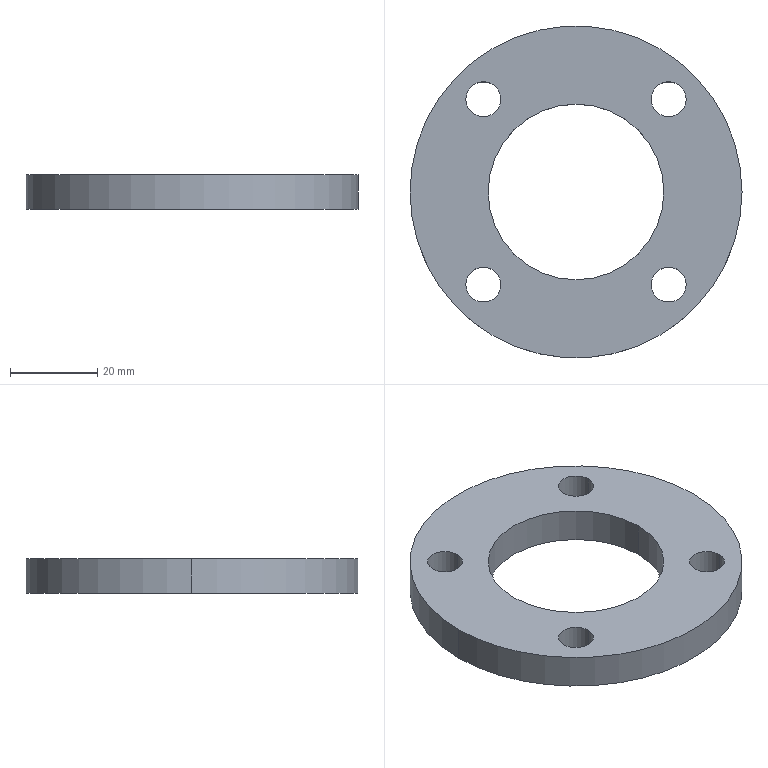Part | SolidWorks | features BaseBody 1 | 1 solid | 14 faces | box 76 x 76 x 8 mm | volume 24529 mm3 | cylinder 12 | plane 2 | commonest cylinder face diameters 8 x8 40.2 x2 76 x2
STEP:
#1=CARTESIAN_POINT('',(-25.213,-21.213,-8.));
#2=VERTEX_POINT('',#1);
#3=CARTESIAN_POINT('',(-25.213,-21.213,0.));
#4=VERTEX_POINT('',#3);
#5=CARTESIAN_POINT('',(-25.213,-21.213,-8.));
#6=DIRECTION('',(0.,0.,1.));
#7=VECTOR('',#6,1000.);
#8=LINE('',#5,#7);
#9=EDGE_CURVE('',#2,#4,#8,.T.);
#10=ORIENTED_EDGE('',*,*,#9,.F.);
#11=CARTESIAN_POINT('',(-17.213,-21.213,-8.));
#12=VERTEX_POINT('',#11);
#13=CARTESIAN_POINT('',(-21.213,-21.213,-8.));
#14=DIRECTION('',(0.,0.,1.));
#15=DIRECTION('',(1.,0.,0.));
#16=AXIS2_PLACEMENT_3D('',#13,#14,#15);
#17=CIRCLE('',#16,4.);
#18=EDGE_CURVE('',#12,#2,#17,.T.);
#19=ORIENTED_EDGE('',*,*,#18,.F.);
#20=CARTESIAN_POINT('',(-17.213,-21.213,0.));
#21=VERTEX_POINT('',#20);
#22=CARTESIAN_POINT('',(-17.213,-21.213,-8.));
#23=DIRECTION('',(0.,0.,1.));
#24=VECTOR('',#23,1000.);
#25=LINE('',#22,#24);
#26=EDGE_CURVE('',#12,#21,#25,.T.);
#27=ORIENTED_EDGE('',*,*,#26,.T.);
#28=CARTESIAN_POINT('',(-21.213,-21.213,0.));
#29=DIRECTION('',(0.,0.,1.));
#30=DIRECTION('',(1.,0.,0.));
#31=AXIS2_PLACEMENT_3D('',#28,#29,#30);
#32=CIRCLE('',#31,4.);
#33=EDGE_CURVE('',#21,#4,#32,.T.);
#34=ORIENTED_EDGE('',*,*,#33,.T.);
#35=EDGE_LOOP('',(#10,#19,#27,#34));
#36=FACE_OUTER_BOUND('',#35,.T.);
#37=CARTESIAN_POINT('',(-21.213,-21.213,-8.));
#38=DIRECTION('',(0.,0.,1.));
#39=DIRECTION('',(1.,0.,0.));
#40=AXIS2_PLACEMENT_3D('',#37,#38,#39);
#41=CYLINDRICAL_SURFACE('',#40,4.);
#42=ADVANCED_FACE('',(#36),#41,.F.);
#43=CARTESIAN_POINT('',(17.213,-21.213,-8.));
#44=VERTEX_POINT('',#43);
#45=CARTESIAN_POINT('',(17.213,-21.213,0.));
#46=VERTEX_POINT('',#45);
#47=CARTESIAN_POINT('',(17.213,-21.213,-8.));
#48=DIRECTION('',(0.,0.,1.));
#49=VECTOR('',#48,1000.);
#50=LINE('',#47,#49);
#51=EDGE_CURVE('',#44,#46,#50,.T.);
#52=ORIENTED_EDGE('',*,*,#51,.F.);
#53=CARTESIAN_POINT('',(25.213,-21.213,-8.));
#54=VERTEX_POINT('',#53);
#55=CARTESIAN_POINT('',(21.213,-21.213,-8.));
#56=DIRECTION('',(0.,0.,1.));
#57=DIRECTION('',(1.,0.,0.));
#58=AXIS2_PLACEMENT_3D('',#55,#56,#57);
#59=CIRCLE('',#58,4.);
#60=EDGE_CURVE('',#54,#44,#59,.T.);
#61=ORIENTED_EDGE('',*,*,#60,.F.);
#62=CARTESIAN_POINT('',(25.213,-21.213,0.));
#63=VERTEX_POINT('',#62);
#64=CARTESIAN_POINT('',(25.213,-21.213,-8.));
#65=DIRECTION('',(0.,0.,1.));
#66=VECTOR('',#65,1000.);
#67=LINE('',#64,#66);
#68=EDGE_CURVE('',#54,#63,#67,.T.);
#69=ORIENTED_EDGE('',*,*,#68,.T.);
#70=CARTESIAN_POINT('',(21.213,-21.213,0.));
#71=DIRECTION('',(0.,0.,1.));
#72=DIRECTION('',(1.,0.,0.));
#73=AXIS2_PLACEMENT_3D('',#70,#71,#72);
#74=CIRCLE('',#73,4.);
#75=EDGE_CURVE('',#63,#46,#74,.T.);
#76=ORIENTED_EDGE('',*,*,#75,.T.);
#77=EDGE_LOOP('',(#52,#61,#69,#76));
#78=FACE_OUTER_BOUND('',#77,.T.);
#79=CARTESIAN_POINT('',(21.213,-21.213,-8.));
#80=DIRECTION('',(0.,0.,1.));
#81=DIRECTION('',(1.,0.,0.));
#82=AXIS2_PLACEMENT_3D('',#79,#80,#81);
#83=CYLINDRICAL_SURFACE('',#82,4.);
#84=ADVANCED_FACE('',(#78),#83,.F.);
#85=CARTESIAN_POINT('',(17.213,21.213,-8.));
#86=VERTEX_POINT('',#85);
#87=CARTESIAN_POINT('',(17.213,21.213,0.));
#88=VERTEX_POINT('',#87);
#89=CARTESIAN_POINT('',(17.213,21.213,-8.));
#90=DIRECTION('',(0.,0.,1.));
#91=VECTOR('',#90,1000.);
#92=LINE('',#89,#91);
#93=EDGE_CURVE('',#86,#88,#92,.T.);
#94=ORIENTED_EDGE('',*,*,#93,.F.);
#95=CARTESIAN_POINT('',(25.213,21.213,-8.));
#96=VERTEX_POINT('',#95);
#97=CARTESIAN_POINT('',(21.213,21.213,-8.));
#98=DIRECTION('',(0.,0.,1.));
#99=DIRECTION('',(1.,0.,0.));
#100=AXIS2_PLACEMENT_3D('',#97,#98,#99);
#101=CIRCLE('',#100,4.);
#102=EDGE_CURVE('',#96,#86,#101,.T.);
#103=ORIENTED_EDGE('',*,*,#102,.F.);
#104=CARTESIAN_POINT('',(25.213,21.213,0.));
#105=VERTEX_POINT('',#104);
#106=CARTESIAN_POINT('',(25.213,21.213,-8.));
#107=DIRECTION('',(0.,0.,1.));
#108=VECTOR('',#107,1000.);
#109=LINE('',#106,#108);
#110=EDGE_CURVE('',#96,#105,#109,.T.);
#111=ORIENTED_EDGE('',*,*,#110,.T.);
#112=CARTESIAN_POINT('',(21.213,21.213,0.));
#113=DIRECTION('',(0.,0.,1.));
#114=DIRECTION('',(1.,0.,0.));
#115=AXIS2_PLACEMENT_3D('',#112,#113,#114);
#116=CIRCLE('',#115,4.);
#117=EDGE_CURVE('',#105,#88,#116,.T.);
#118=ORIENTED_EDGE('',*,*,#117,.T.);
#119=EDGE_LOOP('',(#94,#103,#111,#118));
#120=FACE_OUTER_BOUND('',#119,.T.);
#121=CARTESIAN_POINT('',(21.213,21.213,-8.));
#122=DIRECTION('',(0.,0.,1.));
#123=DIRECTION('',(1.,0.,0.));
#124=AXIS2_PLACEMENT_3D('',#121,#122,#123);
#125=CYLINDRICAL_SURFACE('',#124,4.);
#126=ADVANCED_FACE('',(#120),#125,.F.);
#127=CARTESIAN_POINT('',(-25.213,21.213,-8.));
#128=VERTEX_POINT('',#127);
#129=CARTESIAN_POINT('',(-25.213,21.213,0.));
#130=VERTEX_POINT('',#129);
#131=CARTESIAN_POINT('',(-25.213,21.213,-8.));
#132=DIRECTION('',(0.,0.,1.));
#133=VECTOR('',#132,1000.);
#134=LINE('',#131,#133);
#135=EDGE_CURVE('',#128,#130,#134,.T.);
#136=ORIENTED_EDGE('',*,*,#135,.F.);
#137=CARTESIAN_POINT('',(-17.213,21.213,-8.));
#138=VERTEX_POINT('',#137);
#139=CARTESIAN_POINT('',(-21.213,21.213,-8.));
#140=DIRECTION('',(0.,0.,1.));
#141=DIRECTION('',(1.,0.,0.));
#142=AXIS2_PLACEMENT_3D('',#139,#140,#141);
#143=CIRCLE('',#142,4.);
#144=EDGE_CURVE('',#138,#128,#143,.T.);
#145=ORIENTED_EDGE('',*,*,#144,.F.);
#146=CARTESIAN_POINT('',(-17.213,21.213,0.));
#147=VERTEX_POINT('',#146);
#148=CARTESIAN_POINT('',(-17.213,21.213,-8.));
#149=DIRECTION('',(0.,0.,1.));
#150=VECTOR('',#149,1000.);
#151=LINE('',#148,#150);
#152=EDGE_CURVE('',#138,#147,#151,.T.);
#153=ORIENTED_EDGE('',*,*,#152,.T.);
#154=CARTESIAN_POINT('',(-21.213,21.213,0.));
#155=DIRECTION('',(0.,0.,1.));
#156=DIRECTION('',(1.,0.,0.));
#157=AXIS2_PLACEMENT_3D('',#154,#155,#156);
#158=CIRCLE('',#157,4.);
#159=EDGE_CURVE('',#147,#130,#158,.T.);
#160=ORIENTED_EDGE('',*,*,#159,.T.);
#161=EDGE_LOOP('',(#136,#145,#153,#160));
#162=FACE_OUTER_BOUND('',#161,.T.);
#163=CARTESIAN_POINT('',(-21.213,21.213,-8.));
#164=DIRECTION('',(0.,0.,1.));
#165=DIRECTION('',(1.,0.,0.));
#166=AXIS2_PLACEMENT_3D('',#163,#164,#165);
#167=CYLINDRICAL_SURFACE('',#166,4.);
#168=ADVANCED_FACE('',(#162),#167,.F.);
#169=CARTESIAN_POINT('',(-20.1,0.,-8.));
#170=VERTEX_POINT('',#169);
#171=CARTESIAN_POINT('',(-20.1,0.,0.));
#172=VERTEX_POINT('',#171);
#173=CARTESIAN_POINT('',(-20.1,0.,-8.));
#174=DIRECTION('',(0.,0.,1.));
#175=VECTOR('',#174,1000.);
#176=LINE('',#173,#175);
#177=EDGE_CURVE('',#170,#172,#176,.T.);
#178=ORIENTED_EDGE('',*,*,#177,.F.);
#179=CARTESIAN_POINT('',(20.1,0.,-8.));
#180=VERTEX_POINT('',#179);
#181=CARTESIAN_POINT('',(0.,0.,-8.));
#182=DIRECTION('',(0.,0.,1.));
#183=DIRECTION('',(1.,0.,0.));
#184=AXIS2_PLACEMENT_3D('',#181,#182,#183);
#185=CIRCLE('',#184,20.1);
#186=EDGE_CURVE('',#180,#170,#185,.T.);
#187=ORIENTED_EDGE('',*,*,#186,.F.);
#188=CARTESIAN_POINT('',(20.1,0.,0.));
#189=VERTEX_POINT('',#188);
#190=CARTESIAN_POINT('',(20.1,0.,-8.));
#191=DIRECTION('',(0.,0.,1.));
#192=VECTOR('',#191,1000.);
#193=LINE('',#190,#192);
#194=EDGE_CURVE('',#180,#189,#193,.T.);
#195=ORIENTED_EDGE('',*,*,#194,.T.);
#196=CARTESIAN_POINT('',(0.,0.,0.));
#197=DIRECTION('',(0.,0.,1.));
#198=DIRECTION('',(1.,0.,0.));
#199=AXIS2_PLACEMENT_3D('',#196,#197,#198);
#200=CIRCLE('',#199,20.1);
#201=EDGE_CURVE('',#189,#172,#200,.T.);
#202=ORIENTED_EDGE('',*,*,#201,.T.);
#203=EDGE_LOOP('',(#178,#187,#195,#202));
#204=FACE_OUTER_BOUND('',#203,.T.);
#205=CARTESIAN_POINT('',(0.,0.,-8.));
#206=DIRECTION('',(0.,0.,1.));
#207=DIRECTION('',(1.,0.,0.));
#208=AXIS2_PLACEMENT_3D('',#205,#206,#207);
#209=CYLINDRICAL_SURFACE('',#208,20.1);
#210=ADVANCED_FACE('',(#204),#209,.F.);
#211=ORIENTED_EDGE('',*,*,#201,.F.);
#212=CARTESIAN_POINT('',(0.,0.,0.));
#213=DIRECTION('',(0.,0.,1.));
#214=DIRECTION('',(1.,0.,0.));
#215=AXIS2_PLACEMENT_3D('',#212,#213,#214);
#216=CIRCLE('',#215,20.1);
#217=EDGE_CURVE('',#172,#189,#216,.T.);
#218=ORIENTED_EDGE('',*,*,#217,.F.);
#219=EDGE_LOOP('',(#211,#218));
#220=FACE_BOUND('',#219,.T.);
#221=ORIENTED_EDGE('',*,*,#159,.F.);
#222=CARTESIAN_POINT('',(-21.213,21.213,0.));
#223=DIRECTION('',(0.,0.,1.));
#224=DIRECTION('',(1.,0.,0.));
#225=AXIS2_PLACEMENT_3D('',#222,#223,#224);
#226=CIRCLE('',#225,4.);
#227=EDGE_CURVE('',#130,#147,#226,.T.);
#228=ORIENTED_EDGE('',*,*,#227,.F.);
#229=EDGE_LOOP('',(#221,#228));
#230=FACE_BOUND('',#229,.T.);
#231=ORIENTED_EDGE('',*,*,#117,.F.);
#232=CARTESIAN_POINT('',(21.213,21.213,0.));
#233=DIRECTION('',(0.,0.,1.));
#234=DIRECTION('',(1.,0.,0.));
#235=AXIS2_PLACEMENT_3D('',#232,#233,#234);
#236=CIRCLE('',#235,4.);
#237=EDGE_CURVE('',#88,#105,#236,.T.);
#238=ORIENTED_EDGE('',*,*,#237,.F.);
#239=EDGE_LOOP('',(#231,#238));
#240=FACE_BOUND('',#239,.T.);
#241=ORIENTED_EDGE('',*,*,#75,.F.);
#242=CARTESIAN_POINT('',(21.213,-21.213,0.));
#243=DIRECTION('',(0.,0.,1.));
#244=DIRECTION('',(1.,0.,0.));
#245=AXIS2_PLACEMENT_3D('',#242,#243,#244);
#246=CIRCLE('',#245,4.);
#247=EDGE_CURVE('',#46,#63,#246,.T.);
#248=ORIENTED_EDGE('',*,*,#247,.F.);
#249=EDGE_LOOP('',(#241,#248));
#250=FACE_BOUND('',#249,.T.);
#251=ORIENTED_EDGE('',*,*,#33,.F.);
#252=CARTESIAN_POINT('',(-21.213,-21.213,0.));
#253=DIRECTION('',(0.,0.,1.));
#254=DIRECTION('',(1.,0.,0.));
#255=AXIS2_PLACEMENT_3D('',#252,#253,#254);
#256=CIRCLE('',#255,4.);
#257=EDGE_CURVE('',#4,#21,#256,.T.);
#258=ORIENTED_EDGE('',*,*,#257,.F.);
#259=EDGE_LOOP('',(#251,#258));
#260=FACE_BOUND('',#259,.T.);
#261=CARTESIAN_POINT('',(38.,0.,0.));
#262=VERTEX_POINT('',#261);
#263=CARTESIAN_POINT('',(-38.,0.,0.));
#264=VERTEX_POINT('',#263);
#265=CARTESIAN_POINT('',(0.,0.,0.));
#266=DIRECTION('',(0.,0.,1.));
#267=DIRECTION('',(1.,0.,0.));
#268=AXIS2_PLACEMENT_3D('',#265,#266,#267);
#269=CIRCLE('',#268,38.);
#270=EDGE_CURVE('',#262,#264,#269,.T.);
#271=ORIENTED_EDGE('',*,*,#270,.T.);
#272=CARTESIAN_POINT('',(0.,0.,0.));
#273=DIRECTION('',(0.,0.,1.));
#274=DIRECTION('',(1.,0.,0.));
#275=AXIS2_PLACEMENT_3D('',#272,#273,#274);
#276=CIRCLE('',#275,38.);
#277=EDGE_CURVE('',#264,#262,#276,.T.);
#278=ORIENTED_EDGE('',*,*,#277,.T.);
#279=EDGE_LOOP('',(#271,#278));
#280=FACE_OUTER_BOUND('',#279,.T.);
#281=CARTESIAN_POINT('',(0.,0.,0.));
#282=DIRECTION('',(0.,0.,1.));
#283=DIRECTION('',(1.,0.,0.));
#284=AXIS2_PLACEMENT_3D('',#281,#282,#283);
#285=PLANE('',#284);
#286=ADVANCED_FACE('',(#220,#230,#240,#250,#260,#280),#285,.T.);
#287=ORIENTED_EDGE('',*,*,#186,.T.);
#288=CARTESIAN_POINT('',(0.,0.,-8.));
#289=DIRECTION('',(0.,0.,1.));
#290=DIRECTION('',(1.,0.,0.));
#291=AXIS2_PLACEMENT_3D('',#288,#289,#290);
#292=CIRCLE('',#291,20.1);
#293=EDGE_CURVE('',#170,#180,#292,.T.);
#294=ORIENTED_EDGE('',*,*,#293,.T.);
#295=EDGE_LOOP('',(#287,#294));
#296=FACE_BOUND('',#295,.T.);
#297=ORIENTED_EDGE('',*,*,#144,.T.);
#298=CARTESIAN_POINT('',(-21.213,21.213,-8.));
#299=DIRECTION('',(0.,0.,1.));
#300=DIRECTION('',(1.,0.,0.));
#301=AXIS2_PLACEMENT_3D('',#298,#299,#300);
#302=CIRCLE('',#301,4.);
#303=EDGE_CURVE('',#128,#138,#302,.T.);
#304=ORIENTED_EDGE('',*,*,#303,.T.);
#305=EDGE_LOOP('',(#297,#304));
#306=FACE_BOUND('',#305,.T.);
#307=ORIENTED_EDGE('',*,*,#102,.T.);
#308=CARTESIAN_POINT('',(21.213,21.213,-8.));
#309=DIRECTION('',(0.,0.,1.));
#310=DIRECTION('',(1.,0.,0.));
#311=AXIS2_PLACEMENT_3D('',#308,#309,#310);
#312=CIRCLE('',#311,4.);
#313=EDGE_CURVE('',#86,#96,#312,.T.);
#314=ORIENTED_EDGE('',*,*,#313,.T.);
#315=EDGE_LOOP('',(#307,#314));
#316=FACE_BOUND('',#315,.T.);
#317=ORIENTED_EDGE('',*,*,#60,.T.);
#318=CARTESIAN_POINT('',(21.213,-21.213,-8.));
#319=DIRECTION('',(0.,0.,1.));
#320=DIRECTION('',(1.,0.,0.));
#321=AXIS2_PLACEMENT_3D('',#318,#319,#320);
#322=CIRCLE('',#321,4.);
#323=EDGE_CURVE('',#44,#54,#322,.T.);
#324=ORIENTED_EDGE('',*,*,#323,.T.);
#325=EDGE_LOOP('',(#317,#324));
#326=FACE_BOUND('',#325,.T.);
#327=ORIENTED_EDGE('',*,*,#18,.T.);
#328=CARTESIAN_POINT('',(-21.213,-21.213,-8.));
#329=DIRECTION('',(0.,0.,1.));
#330=DIRECTION('',(1.,0.,0.));
#331=AXIS2_PLACEMENT_3D('',#328,#329,#330);
#332=CIRCLE('',#331,4.);
#333=EDGE_CURVE('',#2,#12,#332,.T.);
#334=ORIENTED_EDGE('',*,*,#333,.T.);
#335=EDGE_LOOP('',(#327,#334));
#336=FACE_BOUND('',#335,.T.);
#337=CARTESIAN_POINT('',(38.,0.,-8.));
#338=VERTEX_POINT('',#337);
#339=CARTESIAN_POINT('',(-38.,0.,-8.));
#340=VERTEX_POINT('',#339);
#341=CARTESIAN_POINT('',(0.,0.,-8.));
#342=DIRECTION('',(0.,0.,1.));
#343=DIRECTION('',(1.,0.,0.));
#344=AXIS2_PLACEMENT_3D('',#341,#342,#343);
#345=CIRCLE('',#344,38.);
#346=EDGE_CURVE('',#338,#340,#345,.T.);
#347=ORIENTED_EDGE('',*,*,#346,.F.);
#348=CARTESIAN_POINT('',(0.,0.,-8.));
#349=DIRECTION('',(0.,0.,1.));
#350=DIRECTION('',(1.,0.,0.));
#351=AXIS2_PLACEMENT_3D('',#348,#349,#350);
#352=CIRCLE('',#351,38.);
#353=EDGE_CURVE('',#340,#338,#352,.T.);
#354=ORIENTED_EDGE('',*,*,#353,.F.);
#355=EDGE_LOOP('',(#347,#354));
#356=FACE_OUTER_BOUND('',#355,.T.);
#357=CARTESIAN_POINT('',(0.,0.,-8.));
#358=DIRECTION('',(0.,0.,1.));
#359=DIRECTION('',(1.,0.,0.));
#360=AXIS2_PLACEMENT_3D('',#357,#358,#359);
#361=PLANE('',#360);
#362=ADVANCED_FACE('',(#296,#306,#316,#326,#336,#356),#361,.F.);
#363=CARTESIAN_POINT('',(-38.,0.,-8.));
#364=DIRECTION('',(0.,0.,1.));
#365=VECTOR('',#364,1000.);
#366=LINE('',#363,#365);
#367=EDGE_CURVE('',#340,#264,#366,.T.);
#368=ORIENTED_EDGE('',*,*,#367,.F.);
#369=ORIENTED_EDGE('',*,*,#353,.T.);
#370=CARTESIAN_POINT('',(38.,0.,-8.));
#371=DIRECTION('',(0.,0.,1.));
#372=VECTOR('',#371,1000.);
#373=LINE('',#370,#372);
#374=EDGE_CURVE('',#338,#262,#373,.T.);
#375=ORIENTED_EDGE('',*,*,#374,.T.);
#376=ORIENTED_EDGE('',*,*,#277,.F.);
#377=EDGE_LOOP('',(#368,#369,#375,#376));
#378=FACE_OUTER_BOUND('',#377,.T.);
#379=CARTESIAN_POINT('',(0.,0.,-8.));
#380=DIRECTION('',(0.,0.,1.));
#381=DIRECTION('',(1.,0.,0.));
#382=AXIS2_PLACEMENT_3D('',#379,#380,#381);
#383=CYLINDRICAL_SURFACE('',#382,38.);
#384=ADVANCED_FACE('',(#378),#383,.T.);
#385=ORIENTED_EDGE('',*,*,#346,.T.);
#386=ORIENTED_EDGE('',*,*,#367,.T.);
#387=ORIENTED_EDGE('',*,*,#270,.F.);
#388=ORIENTED_EDGE('',*,*,#374,.F.);
#389=EDGE_LOOP('',(#385,#386,#387,#388));
#390=FACE_OUTER_BOUND('',#389,.T.);
#391=CARTESIAN_POINT('',(0.,0.,-8.));
#392=DIRECTION('',(0.,0.,1.));
#393=DIRECTION('',(1.,0.,0.));
#394=AXIS2_PLACEMENT_3D('',#391,#392,#393);
#395=CYLINDRICAL_SURFACE('',#394,38.);
#396=ADVANCED_FACE('',(#390),#395,.T.);
#397=ORIENTED_EDGE('',*,*,#293,.F.);
#398=ORIENTED_EDGE('',*,*,#177,.T.);
#399=ORIENTED_EDGE('',*,*,#217,.T.);
#400=ORIENTED_EDGE('',*,*,#194,.F.);
#401=EDGE_LOOP('',(#397,#398,#399,#400));
#402=FACE_OUTER_BOUND('',#401,.T.);
#403=CARTESIAN_POINT('',(0.,0.,-8.));
#404=DIRECTION('',(0.,0.,1.));
#405=DIRECTION('',(1.,0.,0.));
#406=AXIS2_PLACEMENT_3D('',#403,#404,#405);
#407=CYLINDRICAL_SURFACE('',#406,20.1);
#408=ADVANCED_FACE('',(#402),#407,.F.);
#409=ORIENTED_EDGE('',*,*,#303,.F.);
#410=ORIENTED_EDGE('',*,*,#135,.T.);
#411=ORIENTED_EDGE('',*,*,#227,.T.);
#412=ORIENTED_EDGE('',*,*,#152,.F.);
#413=EDGE_LOOP('',(#409,#410,#411,#412));
#414=FACE_OUTER_BOUND('',#413,.T.);
#415=CARTESIAN_POINT('',(-21.213,21.213,-8.));
#416=DIRECTION('',(0.,0.,1.));
#417=DIRECTION('',(1.,0.,0.));
#418=AXIS2_PLACEMENT_3D('',#415,#416,#417);
#419=CYLINDRICAL_SURFACE('',#418,4.);
#420=ADVANCED_FACE('',(#414),#419,.F.);
#421=ORIENTED_EDGE('',*,*,#313,.F.);
#422=ORIENTED_EDGE('',*,*,#93,.T.);
#423=ORIENTED_EDGE('',*,*,#237,.T.);
#424=ORIENTED_EDGE('',*,*,#110,.F.);
#425=EDGE_LOOP('',(#421,#422,#423,#424));
#426=FACE_OUTER_BOUND('',#425,.T.);
#427=CARTESIAN_POINT('',(21.213,21.213,-8.));
#428=DIRECTION('',(0.,0.,1.));
#429=DIRECTION('',(1.,0.,0.));
#430=AXIS2_PLACEMENT_3D('',#427,#428,#429);
#431=CYLINDRICAL_SURFACE('',#430,4.);
#432=ADVANCED_FACE('',(#426),#431,.F.);
#433=ORIENTED_EDGE('',*,*,#323,.F.);
#434=ORIENTED_EDGE('',*,*,#51,.T.);
#435=ORIENTED_EDGE('',*,*,#247,.T.);
#436=ORIENTED_EDGE('',*,*,#68,.F.);
#437=EDGE_LOOP('',(#433,#434,#435,#436));
#438=FACE_OUTER_BOUND('',#437,.T.);
#439=CARTESIAN_POINT('',(21.213,-21.213,-8.));
#440=DIRECTION('',(0.,0.,1.));
#441=DIRECTION('',(1.,0.,0.));
#442=AXIS2_PLACEMENT_3D('',#439,#440,#441);
#443=CYLINDRICAL_SURFACE('',#442,4.);
#444=ADVANCED_FACE('',(#438),#443,.F.);
#445=ORIENTED_EDGE('',*,*,#333,.F.);
#446=ORIENTED_EDGE('',*,*,#9,.T.);
#447=ORIENTED_EDGE('',*,*,#257,.T.);
#448=ORIENTED_EDGE('',*,*,#26,.F.);
#449=EDGE_LOOP('',(#445,#446,#447,#448));
#450=FACE_OUTER_BOUND('',#449,.T.);
#451=CARTESIAN_POINT('',(-21.213,-21.213,-8.));
#452=DIRECTION('',(0.,0.,1.));
#453=DIRECTION('',(1.,0.,0.));
#454=AXIS2_PLACEMENT_3D('',#451,#452,#453);
#455=CYLINDRICAL_SURFACE('',#454,4.);
#456=ADVANCED_FACE('',(#450),#455,.F.);
#457=CLOSED_SHELL('',(#42,#84,#126,#168,#210,#286,#362,#384,#396,#408,#420,#432,#444,#456));
#458=MANIFOLD_SOLID_BREP('',#457);
#459=CARTESIAN_POINT('',(0.,0.,0.));
#460=DIRECTION('',(0.,0.,1.));
#461=DIRECTION('',(1.,0.,0.));
#462=AXIS2_PLACEMENT_3D('',#459,#460,#461);
#463=(LENGTH_UNIT()NAMED_UNIT(*)SI_UNIT(.MILLI.,.METRE.));
#464=UNCERTAINTY_MEASURE_WITH_UNIT(LENGTH_MEASURE(0.00001),#463,'','');
#465=(NAMED_UNIT(*)PLANE_ANGLE_UNIT()SI_UNIT($,.RADIAN.));
#466=(NAMED_UNIT(*)SI_UNIT($,.STERADIAN.)SOLID_ANGLE_UNIT());
#467=(GEOMETRIC_REPRESENTATION_CONTEXT(3)GLOBAL_UNCERTAINTY_ASSIGNED_CONTEXT((#464))GLOBAL_UNIT_ASSIGNED_CONTEXT((#463,#465,#466))REPRESENTATION_CONTEXT('',''));
#468=ADVANCED_BREP_SHAPE_REPRESENTATION('',(#458,#462),#467);